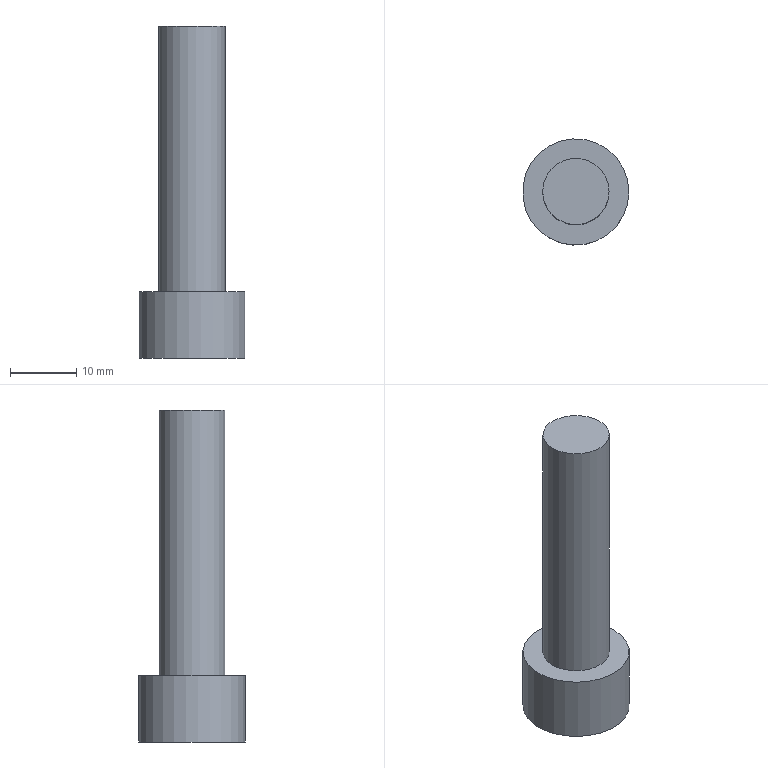Part | NX | features MPPJ 2 | 1 solid | 12 faces | box 16 x 16 x 50 mm | volume 4875 mm3 | plane 10 | cylinder 2 | commonest cylinder face diameters 10 x1 16 x1
STEP:
#1=CARTESIAN_POINT('',(150.5,142.,-269.5));
#2=VERTEX_POINT('',#1);
#3=CARTESIAN_POINT('',(142.5,142.,-269.5));
#4=DIRECTION('',(0.,0.,1.));
#5=DIRECTION('',(1.,0.,0.));
#6=AXIS2_PLACEMENT_3D('',#3,#4,#5);
#7=CIRCLE('',#6,8.);
#8=EDGE_CURVE('',#2,#2,#7,.T.);
#9=ORIENTED_EDGE('',*,*,#8,.F.);
#10=EDGE_LOOP('',(#9));
#11=FACE_BOUND('',#10,.T.);
#12=CARTESIAN_POINT('',(138.5,139.691,-269.5));
#13=VERTEX_POINT('',#12);
#14=CARTESIAN_POINT('',(142.5,137.381,-269.5));
#15=VERTEX_POINT('',#14);
#16=CARTESIAN_POINT('',(138.5,139.691,-269.5));
#17=DIRECTION('',(0.866,-0.5,0.));
#18=VECTOR('',#17,1000.);
#19=LINE('',#16,#18);
#20=EDGE_CURVE('',#13,#15,#19,.T.);
#21=ORIENTED_EDGE('',*,*,#20,.T.);
#22=CARTESIAN_POINT('',(146.5,139.691,-269.5));
#23=VERTEX_POINT('',#22);
#24=CARTESIAN_POINT('',(142.5,137.381,-269.5));
#25=DIRECTION('',(0.866,0.5,0.));
#26=VECTOR('',#25,1000.);
#27=LINE('',#24,#26);
#28=EDGE_CURVE('',#15,#23,#27,.T.);
#29=ORIENTED_EDGE('',*,*,#28,.T.);
#30=CARTESIAN_POINT('',(146.5,144.309,-269.5));
#31=VERTEX_POINT('',#30);
#32=CARTESIAN_POINT('',(146.5,139.691,-269.5));
#33=DIRECTION('',(0.,1.,0.));
#34=VECTOR('',#33,1000.);
#35=LINE('',#32,#34);
#36=EDGE_CURVE('',#23,#31,#35,.T.);
#37=ORIENTED_EDGE('',*,*,#36,.T.);
#38=CARTESIAN_POINT('',(142.5,146.619,-269.5));
#39=VERTEX_POINT('',#38);
#40=CARTESIAN_POINT('',(146.5,144.309,-269.5));
#41=DIRECTION('',(-0.866,0.5,0.));
#42=VECTOR('',#41,1000.);
#43=LINE('',#40,#42);
#44=EDGE_CURVE('',#31,#39,#43,.T.);
#45=ORIENTED_EDGE('',*,*,#44,.T.);
#46=CARTESIAN_POINT('',(138.5,144.309,-269.5));
#47=VERTEX_POINT('',#46);
#48=CARTESIAN_POINT('',(142.5,146.619,-269.5));
#49=DIRECTION('',(-0.866,-0.5,0.));
#50=VECTOR('',#49,1000.);
#51=LINE('',#48,#50);
#52=EDGE_CURVE('',#39,#47,#51,.T.);
#53=ORIENTED_EDGE('',*,*,#52,.T.);
#54=CARTESIAN_POINT('',(138.5,144.309,-269.5));
#55=DIRECTION('',(0.,-1.,0.));
#56=VECTOR('',#55,1000.);
#57=LINE('',#54,#56);
#58=EDGE_CURVE('',#47,#13,#57,.T.);
#59=ORIENTED_EDGE('',*,*,#58,.T.);
#60=EDGE_LOOP('',(#21,#29,#37,#45,#53,#59));
#61=FACE_BOUND('',#60,.T.);
#62=CARTESIAN_POINT('',(142.5,142.,-269.5));
#63=DIRECTION('',(0.,0.,-1.));
#64=DIRECTION('',(-1.,0.,0.));
#65=AXIS2_PLACEMENT_3D('',#62,#63,#64);
#66=PLANE('',#65);
#67=ADVANCED_FACE('',(#11,#61),#66,.T.);
#68=CARTESIAN_POINT('',(147.5,142.,-219.5));
#69=VERTEX_POINT('',#68);
#70=CARTESIAN_POINT('',(142.5,142.,-219.5));
#71=DIRECTION('',(0.,0.,-1.));
#72=DIRECTION('',(1.,0.,0.));
#73=AXIS2_PLACEMENT_3D('',#70,#71,#72);
#74=CIRCLE('',#73,5.);
#75=EDGE_CURVE('',#69,#69,#74,.T.);
#76=ORIENTED_EDGE('',*,*,#75,.F.);
#77=EDGE_LOOP('',(#76));
#78=FACE_BOUND('',#77,.T.);
#79=CARTESIAN_POINT('',(142.5,142.,-219.5));
#80=DIRECTION('',(0.,0.,1.));
#81=DIRECTION('',(1.,0.,0.));
#82=AXIS2_PLACEMENT_3D('',#79,#80,#81);
#83=PLANE('',#82);
#84=ADVANCED_FACE('',(#78),#83,.T.);
#85=CARTESIAN_POINT('',(147.5,142.,-259.5));
#86=VERTEX_POINT('',#85);
#87=CARTESIAN_POINT('',(142.5,142.,-259.5));
#88=DIRECTION('',(0.,0.,1.));
#89=DIRECTION('',(1.,0.,0.));
#90=AXIS2_PLACEMENT_3D('',#87,#88,#89);
#91=CIRCLE('',#90,5.);
#92=EDGE_CURVE('',#86,#86,#91,.F.);
#93=ORIENTED_EDGE('',*,*,#92,.F.);
#94=EDGE_LOOP('',(#93));
#95=FACE_BOUND('',#94,.T.);
#96=ORIENTED_EDGE('',*,*,#75,.T.);
#97=EDGE_LOOP('',(#96));
#98=FACE_BOUND('',#97,.T.);
#99=CARTESIAN_POINT('',(142.5,142.,-269.5));
#100=DIRECTION('',(0.,0.,1.));
#101=DIRECTION('',(1.,0.,0.));
#102=AXIS2_PLACEMENT_3D('',#99,#100,#101);
#103=CYLINDRICAL_SURFACE('',#102,5.);
#104=ADVANCED_FACE('',(#95,#98),#103,.T.);
#105=ORIENTED_EDGE('',*,*,#92,.T.);
#106=EDGE_LOOP('',(#105));
#107=FACE_BOUND('',#106,.T.);
#108=CARTESIAN_POINT('',(150.5,142.,-259.5));
#109=VERTEX_POINT('',#108);
#110=CARTESIAN_POINT('',(142.5,142.,-259.5));
#111=DIRECTION('',(0.,0.,-1.));
#112=DIRECTION('',(1.,0.,0.));
#113=AXIS2_PLACEMENT_3D('',#110,#111,#112);
#114=CIRCLE('',#113,8.);
#115=EDGE_CURVE('',#109,#109,#114,.T.);
#116=ORIENTED_EDGE('',*,*,#115,.F.);
#117=EDGE_LOOP('',(#116));
#118=FACE_BOUND('',#117,.T.);
#119=CARTESIAN_POINT('',(142.5,142.,-259.5));
#120=DIRECTION('',(0.,0.,1.));
#121=DIRECTION('',(1.,0.,0.));
#122=AXIS2_PLACEMENT_3D('',#119,#120,#121);
#123=PLANE('',#122);
#124=ADVANCED_FACE('',(#107,#118),#123,.T.);
#125=ORIENTED_EDGE('',*,*,#115,.T.);
#126=EDGE_LOOP('',(#125));
#127=FACE_BOUND('',#126,.T.);
#128=ORIENTED_EDGE('',*,*,#8,.T.);
#129=EDGE_LOOP('',(#128));
#130=FACE_BOUND('',#129,.T.);
#131=CARTESIAN_POINT('',(142.5,142.,-269.5));
#132=DIRECTION('',(0.,0.,1.));
#133=DIRECTION('',(1.,0.,0.));
#134=AXIS2_PLACEMENT_3D('',#131,#132,#133);
#135=CYLINDRICAL_SURFACE('',#134,8.);
#136=ADVANCED_FACE('',(#127,#130),#135,.T.);
#137=CARTESIAN_POINT('',(142.5,137.381,-264.5));
#138=VERTEX_POINT('',#137);
#139=CARTESIAN_POINT('',(138.5,139.691,-264.5));
#140=VERTEX_POINT('',#139);
#141=CARTESIAN_POINT('',(138.5,139.691,-264.5));
#142=DIRECTION('',(0.866,-0.5,0.));
#143=VECTOR('',#142,1000.);
#144=LINE('',#141,#143);
#145=EDGE_CURVE('',#138,#140,#144,.F.);
#146=ORIENTED_EDGE('',*,*,#145,.F.);
#147=CARTESIAN_POINT('',(142.5,137.381,-269.5));
#148=DIRECTION('',(0.,0.,1.));
#149=VECTOR('',#148,1000.);
#150=LINE('',#147,#149);
#151=EDGE_CURVE('',#138,#15,#150,.F.);
#152=ORIENTED_EDGE('',*,*,#151,.T.);
#153=ORIENTED_EDGE('',*,*,#20,.F.);
#154=CARTESIAN_POINT('',(138.5,139.691,-269.5));
#155=DIRECTION('',(0.,0.,1.));
#156=VECTOR('',#155,1000.);
#157=LINE('',#154,#156);
#158=EDGE_CURVE('',#140,#13,#157,.F.);
#159=ORIENTED_EDGE('',*,*,#158,.F.);
#160=EDGE_LOOP('',(#146,#152,#153,#159));
#161=FACE_BOUND('',#160,.T.);
#162=CARTESIAN_POINT('',(140.5,138.536,-267.));
#163=DIRECTION('',(-0.5,-0.866,0.));
#164=DIRECTION('',(0.866,-0.5,0.));
#165=AXIS2_PLACEMENT_3D('',#162,#163,#164);
#166=PLANE('',#165);
#167=ADVANCED_FACE('',(#161),#166,.F.);
#168=CARTESIAN_POINT('',(138.5,144.309,-264.5));
#169=VERTEX_POINT('',#168);
#170=CARTESIAN_POINT('',(138.5,144.309,-264.5));
#171=DIRECTION('',(0.,-1.,0.));
#172=VECTOR('',#171,1000.);
#173=LINE('',#170,#172);
#174=EDGE_CURVE('',#140,#169,#173,.F.);
#175=ORIENTED_EDGE('',*,*,#174,.F.);
#176=ORIENTED_EDGE('',*,*,#158,.T.);
#177=ORIENTED_EDGE('',*,*,#58,.F.);
#178=CARTESIAN_POINT('',(138.5,144.309,-269.5));
#179=DIRECTION('',(0.,0.,1.));
#180=VECTOR('',#179,1000.);
#181=LINE('',#178,#180);
#182=EDGE_CURVE('',#169,#47,#181,.F.);
#183=ORIENTED_EDGE('',*,*,#182,.F.);
#184=EDGE_LOOP('',(#175,#176,#177,#183));
#185=FACE_BOUND('',#184,.T.);
#186=CARTESIAN_POINT('',(138.5,142.,-267.));
#187=DIRECTION('',(-1.,0.,0.));
#188=DIRECTION('',(0.,0.,1.));
#189=AXIS2_PLACEMENT_3D('',#186,#187,#188);
#190=PLANE('',#189);
#191=ADVANCED_FACE('',(#185),#190,.F.);
#192=CARTESIAN_POINT('',(142.5,146.619,-264.5));
#193=VERTEX_POINT('',#192);
#194=CARTESIAN_POINT('',(142.5,146.619,-264.5));
#195=DIRECTION('',(-0.866,-0.5,0.));
#196=VECTOR('',#195,1000.);
#197=LINE('',#194,#196);
#198=EDGE_CURVE('',#169,#193,#197,.F.);
#199=ORIENTED_EDGE('',*,*,#198,.F.);
#200=ORIENTED_EDGE('',*,*,#182,.T.);
#201=ORIENTED_EDGE('',*,*,#52,.F.);
#202=CARTESIAN_POINT('',(142.5,146.619,-269.5));
#203=DIRECTION('',(0.,0.,1.));
#204=VECTOR('',#203,1000.);
#205=LINE('',#202,#204);
#206=EDGE_CURVE('',#193,#39,#205,.F.);
#207=ORIENTED_EDGE('',*,*,#206,.F.);
#208=EDGE_LOOP('',(#199,#200,#201,#207));
#209=FACE_BOUND('',#208,.T.);
#210=CARTESIAN_POINT('',(140.5,145.464,-267.));
#211=DIRECTION('',(-0.5,0.866,0.));
#212=DIRECTION('',(-0.866,-0.5,0.));
#213=AXIS2_PLACEMENT_3D('',#210,#211,#212);
#214=PLANE('',#213);
#215=ADVANCED_FACE('',(#209),#214,.F.);
#216=CARTESIAN_POINT('',(146.5,144.309,-264.5));
#217=VERTEX_POINT('',#216);
#218=CARTESIAN_POINT('',(146.5,144.309,-264.5));
#219=DIRECTION('',(-0.866,0.5,0.));
#220=VECTOR('',#219,1000.);
#221=LINE('',#218,#220);
#222=EDGE_CURVE('',#193,#217,#221,.F.);
#223=ORIENTED_EDGE('',*,*,#222,.F.);
#224=ORIENTED_EDGE('',*,*,#206,.T.);
#225=ORIENTED_EDGE('',*,*,#44,.F.);
#226=CARTESIAN_POINT('',(146.5,144.309,-269.5));
#227=DIRECTION('',(0.,0.,1.));
#228=VECTOR('',#227,1000.);
#229=LINE('',#226,#228);
#230=EDGE_CURVE('',#217,#31,#229,.F.);
#231=ORIENTED_EDGE('',*,*,#230,.F.);
#232=EDGE_LOOP('',(#223,#224,#225,#231));
#233=FACE_BOUND('',#232,.T.);
#234=CARTESIAN_POINT('',(144.5,145.464,-267.));
#235=DIRECTION('',(0.5,0.866,0.));
#236=DIRECTION('',(-0.866,0.5,0.));
#237=AXIS2_PLACEMENT_3D('',#234,#235,#236);
#238=PLANE('',#237);
#239=ADVANCED_FACE('',(#233),#238,.F.);
#240=CARTESIAN_POINT('',(146.5,139.691,-264.5));
#241=VERTEX_POINT('',#240);
#242=CARTESIAN_POINT('',(146.5,139.691,-264.5));
#243=DIRECTION('',(0.,1.,0.));
#244=VECTOR('',#243,1000.);
#245=LINE('',#242,#244);
#246=EDGE_CURVE('',#217,#241,#245,.F.);
#247=ORIENTED_EDGE('',*,*,#246,.F.);
#248=ORIENTED_EDGE('',*,*,#230,.T.);
#249=ORIENTED_EDGE('',*,*,#36,.F.);
#250=CARTESIAN_POINT('',(146.5,139.691,-269.5));
#251=DIRECTION('',(0.,0.,1.));
#252=VECTOR('',#251,1000.);
#253=LINE('',#250,#252);
#254=EDGE_CURVE('',#241,#23,#253,.F.);
#255=ORIENTED_EDGE('',*,*,#254,.F.);
#256=EDGE_LOOP('',(#247,#248,#249,#255));
#257=FACE_BOUND('',#256,.T.);
#258=CARTESIAN_POINT('',(146.5,142.,-267.));
#259=DIRECTION('',(1.,0.,0.));
#260=DIRECTION('',(0.,0.,-1.));
#261=AXIS2_PLACEMENT_3D('',#258,#259,#260);
#262=PLANE('',#261);
#263=ADVANCED_FACE('',(#257),#262,.F.);
#264=CARTESIAN_POINT('',(142.5,137.381,-264.5));
#265=DIRECTION('',(0.866,0.5,0.));
#266=VECTOR('',#265,1000.);
#267=LINE('',#264,#266);
#268=EDGE_CURVE('',#241,#138,#267,.F.);
#269=ORIENTED_EDGE('',*,*,#268,.F.);
#270=ORIENTED_EDGE('',*,*,#254,.T.);
#271=ORIENTED_EDGE('',*,*,#28,.F.);
#272=ORIENTED_EDGE('',*,*,#151,.F.);
#273=EDGE_LOOP('',(#269,#270,#271,#272));
#274=FACE_BOUND('',#273,.T.);
#275=CARTESIAN_POINT('',(144.5,138.536,-267.));
#276=DIRECTION('',(0.5,-0.866,0.));
#277=DIRECTION('',(0.866,0.5,0.));
#278=AXIS2_PLACEMENT_3D('',#275,#276,#277);
#279=PLANE('',#278);
#280=ADVANCED_FACE('',(#274),#279,.F.);
#281=ORIENTED_EDGE('',*,*,#174,.T.);
#282=ORIENTED_EDGE('',*,*,#198,.T.);
#283=ORIENTED_EDGE('',*,*,#222,.T.);
#284=ORIENTED_EDGE('',*,*,#246,.T.);
#285=ORIENTED_EDGE('',*,*,#268,.T.);
#286=ORIENTED_EDGE('',*,*,#145,.T.);
#287=EDGE_LOOP('',(#281,#282,#283,#284,#285,#286));
#288=FACE_BOUND('',#287,.T.);
#289=CARTESIAN_POINT('',(142.5,142.,-264.5));
#290=DIRECTION('',(0.,0.,1.));
#291=DIRECTION('',(1.,0.,0.));
#292=AXIS2_PLACEMENT_3D('',#289,#290,#291);
#293=PLANE('',#292);
#294=ADVANCED_FACE('',(#288),#293,.F.);
#295=CLOSED_SHELL('',(#67,#84,#104,#124,#136,#167,#191,#215,#239,#263,#280,#294));
#296=MANIFOLD_SOLID_BREP('',#295);
#297=(LENGTH_UNIT()NAMED_UNIT(*)SI_UNIT(.MILLI.,.METRE.));
#298=UNCERTAINTY_MEASURE_WITH_UNIT(LENGTH_MEASURE(0.00001),#297,'','');
#299=(NAMED_UNIT(*)PLANE_ANGLE_UNIT()SI_UNIT($,.RADIAN.));
#300=(NAMED_UNIT(*)SI_UNIT($,.STERADIAN.)SOLID_ANGLE_UNIT());
#301=(GEOMETRIC_REPRESENTATION_CONTEXT(3)GLOBAL_UNCERTAINTY_ASSIGNED_CONTEXT((#298))GLOBAL_UNIT_ASSIGNED_CONTEXT((#297,#299,#300))REPRESENTATION_CONTEXT('',''));
#302=ADVANCED_BREP_SHAPE_REPRESENTATION('',(#296),#301);